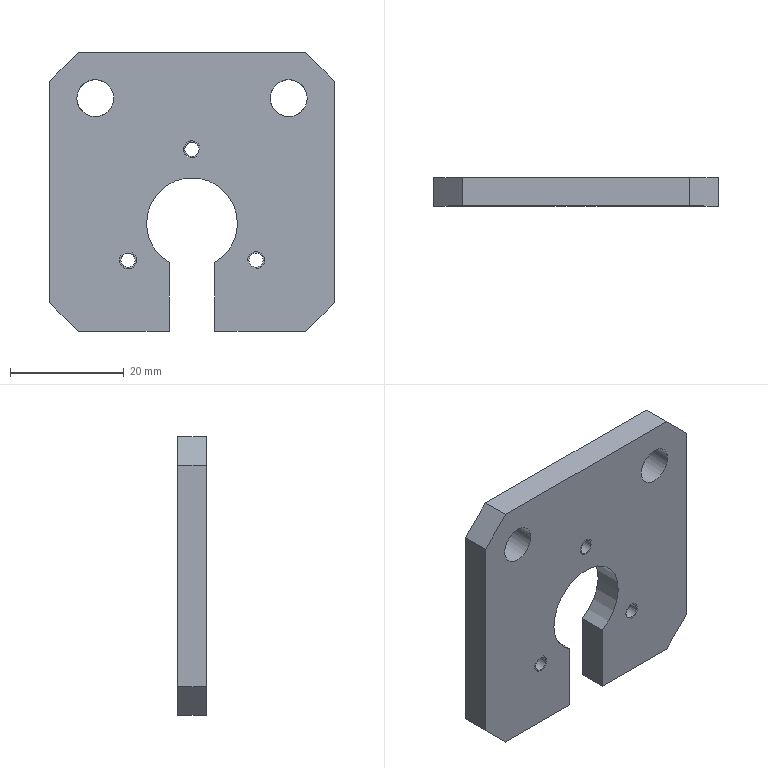Part | STEP file | P011002NM16-000 | 1 solid | 31 faces | box 50 x 5 x 49 mm | volume 10135 mm3 | plane 19 | cylinder 12 | commonest cylinder face diameters 2.5 x3 2.99 x3 3 x3 6.5 x2 16 x1